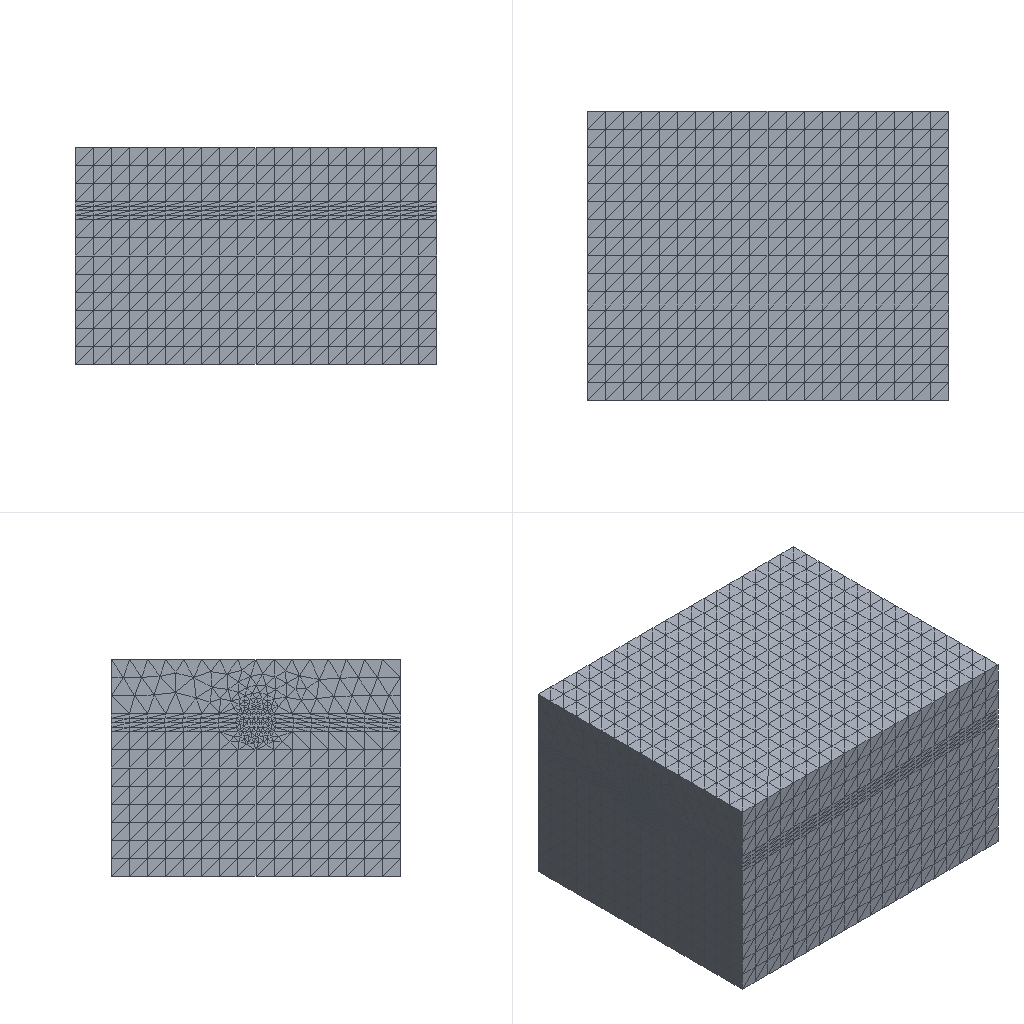Simulation study | abaqus
Set-up summary:
category,name,step,type,value,unit,region
solver,abaqus
solver,version,,,Abaqus/Explicit 3DEXPERIENCE R2017x
units,not stated in the deck,,not stated
analysis,deck,,transient,transient
load_step,Step-1,Step-1,transient
load_step,requested,,,1
mesh,nodes,,,6018
mesh,elements,,,30187
element_type,C3D4,,solid,30187
load,load commands in deck,,count,8
bc,support commands in deck,,count,3
material,LAY1,,in results
material,LAY2,,in results
material,LAY3,,in results
material,LAY4,,in results
check,setup vs results,,match,"per instance, exact: element labels, types and connectivity; labels of the nodes the elements use; coordinates not compared"
Abaqus input file, long lists of numbers shortened:
*Heading
** Job name: Job-1 Model name: Model-1
** Generated by: Abaqus/CAE 2017
*Preprint, echo=NO, model=NO, history=NO, contact=NO
**
** PARTS
**
*Part, name=work
*Node
      1,       15000.,           0.,        6000.
      2,           0.,           0.,        6000.
** (6016 more lines like these left out)
*Element, type=C3D4
   1, 2979, 2980, 2981, 2982
   2, 2980, 2979, 2983, 1466
** (30185 more lines like these left out)
*Nset, nset=Set-6
  23,  24,  25,  26, 160, 162, 427, 428, 484, 485
*Elset, elset=Set-6
   638,  3203,  3239,  3262, 21417, 21426, 21435, 24672, 24681, 24682
*Nset, nset=Set-18
    3,    4,    6,    7,   10,   11,   14,   15,   18,   19,   22,   23,   26,   27,   30,   31
   34,   35,   38,   40,   41,   42,   53,   54,   55,   56,   79,   80,   81,   82,   83,   84
** (116 more lines like these left out)
*Elset, elset=Set-18, generate
 22186,  30187,      1
*Nset, nset=Set-19
    1,    2,    3,    4,    5,    6,    7,    8,    9,   10,   11,   12,   13,   14,   15,   16
   17,   18,   19,   20,   21,   22,   23,   24,   25,   26,   27,   28,   29,   30,   31,   32
** (88 more lines like these left out)
*Elset, elset=Set-19, generate
    1,  4934,     1
*Nset, nset=Set-20
    1,    2,    5,    8,    9,   12,   13,   16,   17,   20,   21,   24,   25,   28,   29,   32
   33,   36,   37,   39,   43,   44,   45,   46,   49,   52,   57,   58,   59,   60,   61,   62
** (55 more lines like these left out)
*Elset, elset=Set-20, generate
 19552,  22185,      1
*Nset, nset=Set-21
   45,   46,   47,   48,   49,   50,   51,   52,  261,  262,  263,  264,  265,  266,  267,  268
  269,  270,  271,  272,  273,  274,  275,  276,  277,  278,  279,  280,  281,  282,  283,  284
** (188 more lines like these left out)
*Elset, elset=Set-21, generate
  4935,  19551,      1
*Elset, elset=_Surf-1_S4, internal
   366,  1986,  2020,  3510,  3818,  4706,  4712,  4733, 19583, 21594, 23987, 24097, 24098
*Elset, elset=_Surf-1_S1, internal
    26,    87,   318,   414,  1525,  1995,  2048,  2434,  3498,  4233,  4422,  4424, 19763, 19809, 24031
*Elset, elset=_Surf-1_S3, internal
     3,    81,   640,   667,   693,   786,  1037,  1656,  1683,  1742,  1743,  1864,  1866,  1913,  1931,  1983
  1989,  1996,  2005,  2006,  2016,  2017,  2024,  2026,  2035,  2038,  2040,  2046,  2055,  2056,  3479,  3512
** (5 more lines like these left out)
*Elset, elset=_Surf-1_S2, internal
  1990,  1997,  2004,  2030,  2051,  3057,  3491,  3509,  3515,  3556,  3660,  4432,  4629, 24055
*Surface, type=ELEMENT, name=Surf-1
_Surf-1_S4, S4
_Surf-1_S1, S1
_Surf-1_S2, S2
_Surf-1_S3, S3
*Elset, elset=_Surf-2_S3, internal
  1838,  1842,  3075,  3078,  3091,  3094,  3102,  3110, 20190, 21354, 24773, 24777, 27476
*Elset, elset=_Surf-2_S4, internal
  1197, 21363
*Elset, elset=_Surf-2_S2, internal
 3080,
*Surface, type=ELEMENT, name=Surf-2
_Surf-2_S3, S3
_Surf-2_S4, S4
_Surf-2_S2, S2
*Elset, elset=_Surf-3_S3, internal
  1711,  3056,  3067,  3121,  3160,  3161,  3951,  3992,  3998, 21355, 21388, 21389, 24505, 24735, 27441
*Elset, elset=_Surf-3_S2, internal
 3145,
*Surface, type=ELEMENT, name=Surf-3
_Surf-3_S3, S3
_Surf-3_S2, S2
*Elset, elset=_Surf-4_S3, internal
  3130,  3155,  3174,  3175,  3180,  3213,  3214,  4144, 21164, 21416, 21432, 24711, 24714, 27595
*Elset, elset=_Surf-4_S4, internal
 1180,
*Elset, elset=_Surf-4_S2, internal
 3205,
*Surface, type=ELEMENT, name=Surf-4
_Surf-4_S3, S3
_Surf-4_S4, S4
_Surf-4_S2, S2
*Elset, elset=_Surf-5_S3, internal
   138,  3243,  3249,  3260,  3262,  3268,  3273, 21426, 21446, 24681, 24682, 24689
*Elset, elset=_Surf-5_S2, internal
 1779, 3265
*Elset, elset=_Surf-5_S4, internal
  1972, 21437
*Surface, type=ELEMENT, name=Surf-5
_Surf-5_S3, S3
_Surf-5_S2, S2
_Surf-5_S4, S4
*Elset, elset=_Surf-6_S3, internal
   668,  1680,  3275,  3281,  3293,  3304,  3311,  3321, 20219, 21471, 21472, 23887, 24651, 27654
*Elset, elset=_Surf-6_S2, internal
 3341,
*Elset, elset=_Surf-6_S4, internal
 4071,
*Surface, type=ELEMENT, name=Surf-6
_Surf-6_S3, S3
_Surf-6_S2, S2
_Surf-6_S4, S4
*Elset, elset=_Surf-7_S3, internal
  2877,  3277,  3333,  3367,  3380,  3384,  3409, 21499, 21500, 21503, 24624, 24638
*Elset, elset=_Surf-7_S2, internal
  3339,  3375, 27840
*Elset, elset=_Surf-7_S4, internal
 3410,
*Surface, type=ELEMENT, name=Surf-7
_Surf-7_S3, S3
_Surf-7_S2, S2
_Surf-7_S4, S4
*Elset, elset=_Surf-8_S1, internal
 22855, 25098
*Elset, elset=_Surf-8_S3, internal
  2648,  2661,  2718,  3269,  3374,  3381,  3395,  3414,  3425, 21518, 21542, 21689, 23998
*Elset, elset=_Surf-8_S2, internal
 2585,
*Surface, type=ELEMENT, name=Surf-8
_Surf-8_S1, S1
_Surf-8_S3, S3
_Surf-8_S2, S2
*Elset, elset=_Surf-9_S3, internal
 22248, 22286, 22303, 22306, 22323, 22325, 22375, 22446, 22610, 22841, 22853, 22861, 23000, 23224, 23505, 23571
 23573, 23589, 23622, 23635, 23646, 23652, 23675, 23681, 23683, 23686, 23708, 23736, 23738, 23747, 23752, 23756
** (68 more lines like these left out)
*Elset, elset=_Surf-9_S2, internal
 22461, 22472, 23879, 23926, 24055, 24312, 24327, 24577, 24917, 25144, 25175, 25352, 25470, 25561, 25592, 25593
 25620, 25667, 25925, 26324, 26512, 26573, 26697, 26790, 26837, 26986, 26996, 27104, 27175, 27361, 27429, 27822
** (1 more lines like these left out)
*Elset, elset=_Surf-9_S1, internal
 22385, 22478, 22496, 23022, 23057, 24031, 24378, 24415, 24577, 24631, 24692, 24826, 24914, 25005, 25036, 25162
 25278, 25452, 25502, 25557, 25592, 26335, 26693, 27009, 27043, 27045, 27058, 27114, 27190, 27229, 27274, 27289
** (1 more lines like these left out)
*Elset, elset=_Surf-9_S4, internal
 22472, 22495, 22723, 22824, 23115, 23862, 23950, 23987, 24097, 24098, 24178, 24269, 24302, 24312, 24378, 24616
 24618, 24713, 24796, 24797, 24812, 24852, 25025, 25279, 25292, 25448, 25487, 25519, 25560, 25585, 25593, 25606
** (2 more lines like these left out)
*Surface, type=ELEMENT, name=Surf-9
_Surf-9_S3, S3
_Surf-9_S2, S2
_Surf-9_S4, S4
_Surf-9_S1, S1
** Section: lay2
*Solid Section, elset=Set-19, material=lay2
,
** Section: lay4
*Solid Section, elset=Set-21, material=lay4
,
** Section: lay3
*Solid Section, elset=Set-20, material=lay3
,
** Section: lay1
*Solid Section, elset=Set-18, material=lay1
,
*End Part
**
**
** ASSEMBLY
**
*Assembly, name=Assembly
**
*Instance, name=work-1, part=work
*End Instance
**
*Node
      1,       15000.,       -6000.,        6375.
*Nset, nset=Set-1, instance=work-1
   47,   48,   50,   51,  282,  283,  284,  285,  286,  287,  288,  289,  290,  291,  292,  293
  294,  295,  296,  328,  329,  330,  331,  332,  333,  334,  335,  336,  337,  338,  339,  340
** (21 more lines like these left out)
*Elset, elset=Set-1, instance=work-1
  5079,  5260,  5351,  5424,  5491,  5549,  5600,  5900,  6122,  6198,  6319,  6540,  6547,  6590,  6631,  6639
  6641,  6653,  6660,  6676,  6682,  6708,  6717,  6723,  6737,  6741,  6757,  6776,  6786,  6848,  6878,  6887
** (38 more lines like these left out)
*Nset, nset=Set-2, instance=work-1
    1,    2,    3,    4,    5,    6,    7,    8,    9,   10,   39,   40,   41,   42,   43,   44
   45,   46,   47,   48,   49,   50,   51,   52,   53,   54,   55,   56,   76,   77,   78,   98
** (38 more lines like these left out)
*Elset, elset=Set-2, instance=work-1
    13,    57,    74,    79,    94,    95,    98,    99,   208,   209,   276,   450,   571,   586,   736,   877
  1336,  1346,  1351,  1358,  1359,  1409,  1414,  1417,  1442,  1462,  1523,  1560,  1571,  1572,  1575,  1577
** (67 more lines like these left out)
*Nset, nset=Set-3, instance=work-1
    1,    2,    3,    4,    9,   10,   39,   40,   45,   46,   47,   48,   49,   50,   51,   52
   53,   54,   55,   56,   57,   58,   59,   60,   61,   62,   63,   64,   65,   66,   67,   68
** (40 more lines like these left out)
*Elset, elset=Set-3, instance=work-1
   108,   110,   111,   114,   115,   121,   123,   184,   186,   187,   192,   324,   357,   435,   702,   933
  1048,  1073,  1113,  1117,  1210,  1221,  1226,  1293,  1434,  1600,  1602,  1607,  1610,  1622,  1626,  1648
** (73 more lines like these left out)
*Nset, nset=Set-4, instance=work-1
    1,    2,    3,    4,    9,   10,   39,   40,   45,   46,   47,   48,   49,   50,   51,   52
   53,   54,   55,   56,   57,   58,   59,   60,   61,   62,   63,   64,   65,   66,   67,   68
** (40 more lines like these left out)
*Elset, elset=Set-4, instance=work-1
   108,   110,   111,   114,   115,   121,   123,   184,   186,   187,   192,   324,   357,   435,   702,   933
  1048,  1073,  1113,  1117,  1210,  1221,  1226,  1293,  1434,  1600,  1602,  1607,  1610,  1622,  1626,  1648
** (73 more lines like these left out)
*Nset, nset=Set-5, instance=work-1
    1,    2,    3,    4,    5,    6,    7,    8,    9,   10,   39,   40,   41,   42,   43,   44
   45,   46,   47,   48,   49,   50,   51,   52,   53,   54,   55,   56,   76,   77,   78,   98
** (38 more lines like these left out)
*Elset, elset=Set-5, instance=work-1
    13,    57,    74,    79,    94,    95,    98,    99,   208,   209,   276,   450,   571,   586,   736,   877
  1336,  1346,  1358,  1359,  1409,  1414,  1417,  1442,  1462,  1523,  1560,  1571,  1572,  1575,  1577,  1578
** (66 more lines like these left out)
*Elset, elset=_Surf-1_S3, internal, instance=work-1
 22303, 22325, 22446, 22861, 23000, 23622, 23646, 23675, 23681, 23683, 23686, 23738, 23747, 23779, 23797, 23808
 23853, 23856, 23866, 23868, 23871, 23874, 23895, 23905, 23909, 23923, 23963, 23978, 23990, 23992, 24005, 24006
** (36 more lines like these left out)
*Elset, elset=_Surf-1_S1, internal, instance=work-1
 22385, 23057, 24378, 24577, 27009, 27043, 27045, 29296
*Elset, elset=_Surf-1_S4, internal, instance=work-1
 22472, 22495, 24312, 24618, 24713, 25025, 25585, 25606, 26185, 26191, 26603, 26840, 26975, 26990, 27598, 28209
 28308, 28790
*Elset, elset=_Surf-1_S2, internal, instance=work-1
 23879, 24327, 25175, 25561, 25620, 25667, 26324, 26573, 26697, 26790, 26986, 26996, 28443, 29731, 29814
*Surface, type=ELEMENT, name=Surf-1
_Surf-1_S3, S3
_Surf-1_S1, S1
_Surf-1_S4, S4
_Surf-1_S2, S2
*Elset, elset=_Surf-5_S4, internal, instance=work-1
   366,  1986,  2020,  3510,  3818,  4706,  4712,  4733, 19583, 21594, 23987, 24097, 24098
*Elset, elset=_Surf-5_S1, internal, instance=work-1
    26,    87,   318,   414,  1525,  1995,  2048,  2434,  3498,  4233,  4422,  4424, 19763, 19809, 24031
*Elset, elset=_Surf-5_S3, internal, instance=work-1
     3,    81,   640,   667,   693,   786,  1037,  1656,  1683,  1742,  1743,  1864,  1866,  1913,  1931,  1983
  1989,  1996,  2005,  2006,  2016,  2017,  2024,  2026,  2035,  2038,  2040,  2046,  2055,  2056,  3479,  3512
** (5 more lines like these left out)
*Elset, elset=_Surf-5_S2, internal, instance=work-1
  1990,  1997,  2004,  2030,  2051,  3057,  3491,  3509,  3515,  3556,  3660,  4432,  4629, 24055
*Surface, type=ELEMENT, name=Surf-5
_Surf-5_S4, S4
_Surf-5_S1, S1
_Surf-5_S2, S2
_Surf-5_S3, S3
*End Assembly
*Amplitude, name=Amp-1
             0.,              1.,              1.,              1.,            1.01,              0.
*Amplitude, name=Amp-2
             0.,              0.,              1.,              0.,              2.,              0.,            2.01,              1.
             3.,              1.,            3.01,              0.
*Amplitude, name=Amp-3
             0.,              0.,              1.,              0.,              3.,              0.,            3.01,              1.
             4.,              1.,            4.01,              0.
*Amplitude, name=Amp-4
             0.,              0.,              1.,              0.,              4.,              0.,            4.01,              1.
             5.,              1.,            5.01,              0.
*Amplitude, name=Amp-5
             0.,              0.,              1.,              0.,              5.,              0.,            5.01,              1.
             6.,              1.,            6.01,              0.
*Amplitude, name=Amp-6
             0.,              0.,              1.,              0.,              6.,              0.,            6.01,              1.
             7.,              1.,            7.01,              0.
*Amplitude, name=Amp-7
             0.,              0.,              1.,              0.,              7.,              0.,            7.01,              1.
             8.,              1.,            8.01,              0.
*Amplitude, name=Amp-8
             0.,              0.,              1.,              0.,              8.,              0.,            8.01,              1.
             9.,              1.,            9.01,              0.
**
** MATERIALS
**
*Material, name=lay1
*Damage Initiation, criterion=SHEAR
 0.0015,0.,0.
*Damage Evolution, type=DISPLACEMENT
 0.1,
*Density
 1.87e-09,
*Drucker Prager
 11.2, 1.,25.
*Drucker Prager Hardening
  290.,      0.
  328.,  0.0007
  582., 0.00122
 107.5, 0.00203
 1342., 0.00244
 1460., 0.00264
 1596., 0.00285
 1859., 0.00326
 2174., 0.00369
 2288., 0.00432
 2302., 0.00451
*Elastic
 3.11, 0.4
*Material, name=lay2
*Damage Initiation, criterion=SHEAR
 0.0025,0.,0.
*Damage Evolution, type=DISPLACEMENT
 0.1,
*Density
 1.92e-09,
*Drucker Prager
 27.5, 1.,36.
*Drucker Prager Hardening
  290.,      0.
  328.,  0.0007
  582., 0.00122
 107.5, 0.00203
 1342., 0.00244
 1460., 0.00264
 1596., 0.00285
 1859., 0.00326
 2174., 0.00369
 2288., 0.00432
 2302., 0.00451
*Elastic
 7.4, 0.3
*Material, name=lay3
*Damage Initiation, criterion=SHEAR
 0.0035,0.,0.
*Damage Evolution, type=DISPLACEMENT
 0.1,
*Density
 1.97e-09,
*Drucker Prager
 17.1, 1.,21.
*Drucker Prager Hardening
  290.,      0.
  328.,  0.0007
  582., 0.00122
 107.5, 0.00203
 1342., 0.00244
 1460., 0.00264
 1596., 0.00285
 1859., 0.00326
 2174., 0.00369
 2288., 0.00432
 2302., 0.00451
*Elastic
 8.5, 0.4
*Material, name=lay4
*Damage Initiation, criterion=SHEAR
 0.0045,0.,0.
*Damage Evolution, type=DISPLACEMENT
 0.1,
*Density
 1.95e-09,
*Drucker Prager
10., 1.,29.
*Drucker Prager Hardening
  290.,      0.
  328.,  0.0007
  582., 0.00122
 107.5, 0.00203
 1342., 0.00244
 1460., 0.00264
 1596., 0.00285
 1859., 0.00326
 2174., 0.00369
 2288., 0.00432
 2302., 0.00451
*Elastic
 7.65, 0.34
**
** BOUNDARY CONDITIONS
**
** Name: BC-1 Type: 对称/反对称/完全固定
*Boundary
Set-1, PINNED
** ----------------------------------------------------------------
**
** STEP: Step-1
**
*Step, name=Step-1, nlgeom=YES
*Dynamic, Explicit
, 9.01
*Bulk Viscosity
0.06, 1.2
** Mass Scaling: Semi-Automatic
**               Whole Model
*Fixed Mass Scaling, factor=100.
**
** BOUNDARY CONDITIONS
**
** Name: BC-2 Type: 位移/转角
*Boundary
Set-4, 2, 2
** Name: BC-3 Type: 位移/转角
*Boundary
Set-5, 1, 1
**
** LOADS
**
** Name: Load-1   Type: Surface traction
*Dsload, amplitude=Amp-1
Surf-5, TRVEC, 0.15, -1., 0., 0.
** Name: Load-1-Copy   Type: Surface traction
*Dsload, amplitude=Amp-2
work-1.Surf-2, TRVEC, 0.15, -1., 0., 0.
** Name: Load-1-Copy-Copy   Type: Surface traction
*Dsload, amplitude=Amp-3
work-1.Surf-3, TRVEC, 0.15, -1., 0., 0.
** Name: Load-1-Copy-Copy-Copy   Type: Surface traction
*Dsload, amplitude=Amp-4
work-1.Surf-4, TRVEC, 0.15, -1., 0., 0.
** Name: Load-1-Copy-Copy-Copy-Copy   Type: Surface traction
*Dsload, amplitude=Amp-5
work-1.Surf-5, TRVEC, 0.15, -1., 0., 0.
** Name: Load-1-Copy-Copy-Copy-Copy-Copy   Type: Surface traction
*Dsload, amplitude=Amp-6
work-1.Surf-6, TRVEC, 0.15, -1., 0., 0.
** Name: Load-1-Copy-Copy-Copy-Copy-Copy-Copy   Type: Surface traction
*Dsload, amplitude=Amp-7
work-1.Surf-7, TRVEC, 0.15, -1., 0., 0.
** Name: Load-8   Type: Surface traction
*Dsload, amplitude=Amp-8
work-1.Surf-8, TRVEC, 0.15, -1., 0., 0.
**
** OUTPUT REQUESTS
**
*Restart, write, number interval=1, time marks=NO
**
** FIELD OUTPUT: F-Output-1
**
*Output, field, number interval=100
*Node Output
A, RF, U, V
*Element Output, directions=YES
E, FV, LE, MFR, MISES, NFORC, PE, PEEQ, PEEQVAVG, PEVAVG, S, SDV, STATUS, UVARM
*Contact Output
CSTRESS,
**
** HISTORY OUTPUT: H-Output-1
**
*Output, history, variable=PRESELECT, time interval=0.0901
*End Step
Results summary:
result,step,Step-1,completed,increments=981 time=9.01/9.01
result,analysis,,,transient
result,last_loadstep,,,1
result,primary field,,,U
result,reaction total,,FX,425000.691,model units
result,reaction total,,FY,-36307.106,model units
result,reaction total,,FZ,25524.801,model units